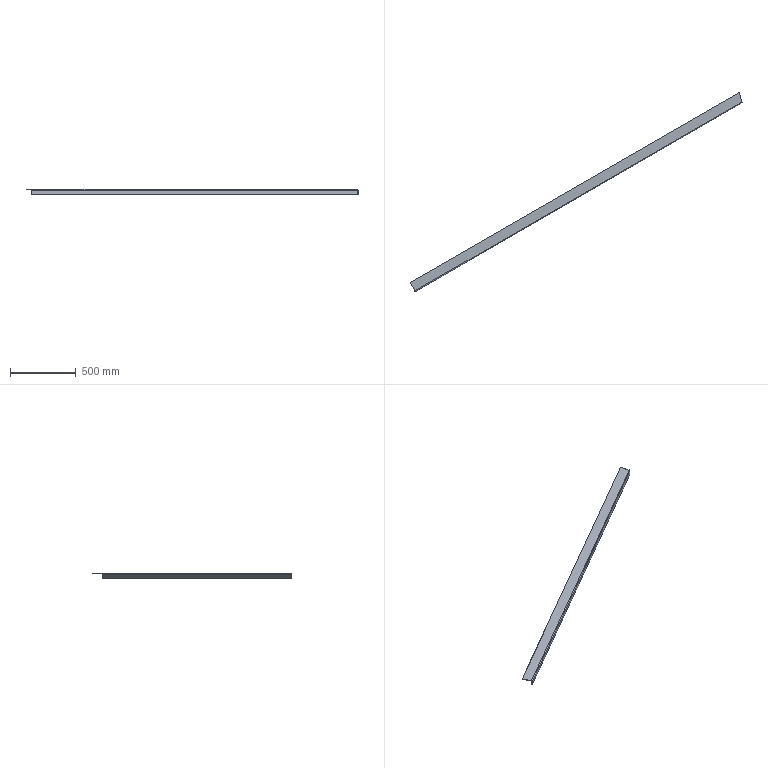Part | SolidWorks | features EdgeFlange 1, FlatPattern 1, ICE 1, SMBaseFlange 1, SheetMetal 1 | 1 solid | 16 faces | box 2517 x 1510 x 40 mm | volume 989838 mm3 | plane 14 | cylinder 2 | commonest cylinder face diameters 6 x1 12 x1
STEP:
#1=CARTESIAN_POINT('',(-2.01,7.5,-3.));
#2=VERTEX_POINT('',#1);
#3=CARTESIAN_POINT('',(-2.01,7.5,0.));
#4=VERTEX_POINT('',#3);
#5=CARTESIAN_POINT('',(-2.01,7.5,-3.));
#6=DIRECTION('',(0.,0.,1.));
#7=VECTOR('',#6,1000.);
#8=LINE('',#5,#7);
#9=EDGE_CURVE('',#2,#4,#8,.T.);
#10=ORIENTED_EDGE('',*,*,#9,.F.);
#11=CARTESIAN_POINT('',(-21.436,80.,-3.));
#12=VERTEX_POINT('',#11);
#13=CARTESIAN_POINT('',(0.,0.,-3.));
#14=DIRECTION('',(-0.2588,0.9659,0.));
#15=VECTOR('',#14,1000.);
#16=LINE('',#13,#15);
#17=EDGE_CURVE('',#2,#12,#16,.T.);
#18=ORIENTED_EDGE('',*,*,#17,.T.);
#19=CARTESIAN_POINT('',(-21.436,80.,0.));
#20=VERTEX_POINT('',#19);
#21=CARTESIAN_POINT('',(-21.436,80.,-3.));
#22=DIRECTION('',(0.,0.,1.));
#23=VECTOR('',#22,1000.);
#24=LINE('',#21,#23);
#25=EDGE_CURVE('',#12,#20,#24,.T.);
#26=ORIENTED_EDGE('',*,*,#25,.T.);
#27=CARTESIAN_POINT('',(0.,0.,0.));
#28=DIRECTION('',(-0.2588,0.9659,0.));
#29=VECTOR('',#28,1000.);
#30=LINE('',#27,#29);
#31=EDGE_CURVE('',#4,#20,#30,.T.);
#32=ORIENTED_EDGE('',*,*,#31,.F.);
#33=EDGE_LOOP('',(#10,#18,#26,#32));
#34=FACE_OUTER_BOUND('',#33,.T.);
#35=CARTESIAN_POINT('',(0.,0.,-3.));
#36=DIRECTION('',(0.9659,0.2588,0.));
#37=DIRECTION('',(-0.2588,0.9659,0.));
#38=AXIS2_PLACEMENT_3D('',#35,#36,#37);
#39=PLANE('',#38);
#40=ADVANCED_FACE('',(#34),#39,.T.);
#41=CARTESIAN_POINT('',(-2516.833,-1360.718,-3.));
#42=VERTEX_POINT('',#41);
#43=CARTESIAN_POINT('',(-2479.833,-1424.804,-3.));
#44=VERTEX_POINT('',#43);
#45=CARTESIAN_POINT('',(-2476.833,-1430.,-3.));
#46=DIRECTION('',(0.5,-0.866,0.));
#47=VECTOR('',#46,1000.);
#48=LINE('',#45,#47);
#49=EDGE_CURVE('',#42,#44,#48,.T.);
#50=ORIENTED_EDGE('',*,*,#49,.T.);
#51=CARTESIAN_POINT('',(-2479.833,-1424.804,0.));
#52=VERTEX_POINT('',#51);
#53=CARTESIAN_POINT('',(-2479.833,-1424.804,-3.));
#54=DIRECTION('',(0.,0.,1.));
#55=VECTOR('',#54,1000.);
#56=LINE('',#53,#55);
#57=EDGE_CURVE('',#44,#52,#56,.T.);
#58=ORIENTED_EDGE('',*,*,#57,.T.);
#59=CARTESIAN_POINT('',(-2516.833,-1360.718,0.));
#60=VERTEX_POINT('',#59);
#61=CARTESIAN_POINT('',(-2476.833,-1430.,0.));
#62=DIRECTION('',(0.5,-0.866,0.));
#63=VECTOR('',#62,1000.);
#64=LINE('',#61,#63);
#65=EDGE_CURVE('',#60,#52,#64,.T.);
#66=ORIENTED_EDGE('',*,*,#65,.F.);
#67=CARTESIAN_POINT('',(-2516.833,-1360.718,-3.));
#68=DIRECTION('',(0.,0.,1.));
#69=VECTOR('',#68,1000.);
#70=LINE('',#67,#69);
#71=EDGE_CURVE('',#42,#60,#70,.T.);
#72=ORIENTED_EDGE('',*,*,#71,.F.);
#73=EDGE_LOOP('',(#50,#58,#66,#72));
#74=FACE_OUTER_BOUND('',#73,.T.);
#75=CARTESIAN_POINT('',(-2476.833,-1430.,-3.));
#76=DIRECTION('',(-0.866,-0.5,0.));
#77=DIRECTION('',(0.5,-0.866,0.));
#78=AXIS2_PLACEMENT_3D('',#75,#76,#77);
#79=PLANE('',#78);
#80=ADVANCED_FACE('',(#74),#79,.T.);
#81=ORIENTED_EDGE('',*,*,#17,.F.);
#82=CARTESIAN_POINT('',(-3.75,6.495,-3.));
#83=VERTEX_POINT('',#82);
#84=CARTESIAN_POINT('',(-3.75,6.495,-3.));
#85=DIRECTION('',(0.866,0.5,0.));
#86=VECTOR('',#85,1000.);
#87=LINE('',#84,#86);
#88=EDGE_CURVE('',#83,#2,#87,.T.);
#89=ORIENTED_EDGE('',*,*,#88,.F.);
#90=CARTESIAN_POINT('',(-3.,5.196,-3.));
#91=VERTEX_POINT('',#90);
#92=CARTESIAN_POINT('',(-3.,5.196,-3.));
#93=DIRECTION('',(-0.5,0.866,0.));
#94=VECTOR('',#93,1000.);
#95=LINE('',#92,#94);
#96=EDGE_CURVE('',#91,#83,#95,.T.);
#97=ORIENTED_EDGE('',*,*,#96,.F.);
#98=CARTESIAN_POINT('',(-2479.833,-1424.804,-3.));
#99=DIRECTION('',(0.866,0.5,0.));
#100=VECTOR('',#99,1000.);
#101=LINE('',#98,#100);
#102=EDGE_CURVE('',#44,#91,#101,.T.);
#103=ORIENTED_EDGE('',*,*,#102,.F.);
#104=ORIENTED_EDGE('',*,*,#49,.F.);
#105=CARTESIAN_POINT('',(-21.436,80.,-3.));
#106=DIRECTION('',(-0.866,-0.5,0.));
#107=VECTOR('',#106,1000.);
#108=LINE('',#105,#107);
#109=EDGE_CURVE('',#12,#42,#108,.T.);
#110=ORIENTED_EDGE('',*,*,#109,.F.);
#111=EDGE_LOOP('',(#81,#89,#97,#103,#104,#110));
#112=FACE_OUTER_BOUND('',#111,.T.);
#113=CARTESIAN_POINT('',(0.,0.,-3.));
#114=DIRECTION('',(0.,0.,1.));
#115=DIRECTION('',(1.,0.,0.));
#116=AXIS2_PLACEMENT_3D('',#113,#114,#115);
#117=PLANE('',#116);
#118=ADVANCED_FACE('',(#112),#117,.F.);
#119=CARTESIAN_POINT('',(-3.75,6.495,0.));
#120=VERTEX_POINT('',#119);
#121=CARTESIAN_POINT('',(-3.75,6.495,0.));
#122=DIRECTION('',(0.866,0.5,0.));
#123=VECTOR('',#122,1000.);
#124=LINE('',#121,#123);
#125=EDGE_CURVE('',#120,#4,#124,.T.);
#126=ORIENTED_EDGE('',*,*,#125,.T.);
#127=ORIENTED_EDGE('',*,*,#31,.T.);
#128=CARTESIAN_POINT('',(-21.436,80.,0.));
#129=DIRECTION('',(-0.866,-0.5,0.));
#130=VECTOR('',#129,1000.);
#131=LINE('',#128,#130);
#132=EDGE_CURVE('',#20,#60,#131,.T.);
#133=ORIENTED_EDGE('',*,*,#132,.T.);
#134=ORIENTED_EDGE('',*,*,#65,.T.);
#135=CARTESIAN_POINT('',(-3.,5.196,0.));
#136=VERTEX_POINT('',#135);
#137=CARTESIAN_POINT('',(-2479.833,-1424.804,0.));
#138=DIRECTION('',(0.866,0.5,0.));
#139=VECTOR('',#138,1000.);
#140=LINE('',#137,#139);
#141=EDGE_CURVE('',#52,#136,#140,.T.);
#142=ORIENTED_EDGE('',*,*,#141,.T.);
#143=CARTESIAN_POINT('',(0.,0.,0.));
#144=DIRECTION('',(-0.5,0.866,0.));
#145=VECTOR('',#144,1000.);
#146=LINE('',#143,#145);
#147=EDGE_CURVE('',#136,#120,#146,.T.);
#148=ORIENTED_EDGE('',*,*,#147,.T.);
#149=EDGE_LOOP('',(#126,#127,#133,#134,#142,#148));
#150=FACE_OUTER_BOUND('',#149,.T.);
#151=CARTESIAN_POINT('',(0.,0.,0.));
#152=DIRECTION('',(0.,0.,1.));
#153=DIRECTION('',(1.,0.,0.));
#154=AXIS2_PLACEMENT_3D('',#151,#152,#153);
#155=PLANE('',#154);
#156=ADVANCED_FACE('',(#150),#155,.T.);
#157=ORIENTED_EDGE('',*,*,#132,.F.);
#158=ORIENTED_EDGE('',*,*,#25,.F.);
#159=ORIENTED_EDGE('',*,*,#109,.T.);
#160=ORIENTED_EDGE('',*,*,#71,.T.);
#161=EDGE_LOOP('',(#157,#158,#159,#160));
#162=FACE_OUTER_BOUND('',#161,.T.);
#163=CARTESIAN_POINT('',(-21.436,80.,-3.));
#164=DIRECTION('',(-0.5,0.866,0.));
#165=DIRECTION('',(-0.866,-0.5,0.));
#166=AXIS2_PLACEMENT_3D('',#163,#164,#165);
#167=PLANE('',#166);
#168=ADVANCED_FACE('',(#162),#167,.T.);
#169=ORIENTED_EDGE('',*,*,#147,.F.);
#170=CARTESIAN_POINT('',(-3.,5.196,-3.));
#171=DIRECTION('',(0.,0.,1.));
#172=VECTOR('',#171,1000.);
#173=LINE('',#170,#172);
#174=EDGE_CURVE('',#91,#136,#173,.T.);
#175=ORIENTED_EDGE('',*,*,#174,.F.);
#176=ORIENTED_EDGE('',*,*,#96,.T.);
#177=CARTESIAN_POINT('',(-3.75,6.495,-3.));
#178=DIRECTION('',(0.,0.,1.));
#179=VECTOR('',#178,1000.);
#180=LINE('',#177,#179);
#181=EDGE_CURVE('',#83,#120,#180,.T.);
#182=ORIENTED_EDGE('',*,*,#181,.T.);
#183=EDGE_LOOP('',(#169,#175,#176,#182));
#184=FACE_OUTER_BOUND('',#183,.T.);
#185=CARTESIAN_POINT('',(-3.,5.196,-3.));
#186=DIRECTION('',(0.866,0.5,0.));
#187=DIRECTION('',(-0.5,0.866,0.));
#188=AXIS2_PLACEMENT_3D('',#185,#186,#187);
#189=PLANE('',#188);
#190=ADVANCED_FACE('',(#184),#189,.T.);
#191=ORIENTED_EDGE('',*,*,#125,.F.);
#192=ORIENTED_EDGE('',*,*,#181,.F.);
#193=ORIENTED_EDGE('',*,*,#88,.T.);
#194=ORIENTED_EDGE('',*,*,#9,.T.);
#195=EDGE_LOOP('',(#191,#192,#193,#194));
#196=FACE_OUTER_BOUND('',#195,.T.);
#197=CARTESIAN_POINT('',(-3.75,6.495,-3.));
#198=DIRECTION('',(0.5,-0.866,0.));
#199=DIRECTION('',(0.866,0.5,0.));
#200=AXIS2_PLACEMENT_3D('',#197,#198,#199);
#201=PLANE('',#200);
#202=ADVANCED_FACE('',(#196),#201,.T.);
#203=CARTESIAN_POINT('',(-1.5,2.598,-6.));
#204=VERTEX_POINT('',#203);
#205=CARTESIAN_POINT('',(0.,0.,-6.));
#206=VERTEX_POINT('',#205);
#207=CARTESIAN_POINT('',(0.,0.,-6.));
#208=DIRECTION('',(0.5,-0.866,0.));
#209=VECTOR('',#208,1000.);
#210=LINE('',#207,#209);
#211=EDGE_CURVE('',#204,#206,#210,.T.);
#212=ORIENTED_EDGE('',*,*,#211,.F.);
#213=CARTESIAN_POINT('',(-3.,5.196,-6.));
#214=DIRECTION('',(0.866,0.5,0.));
#215=DIRECTION('',(0.5,-0.866,0.));
#216=AXIS2_PLACEMENT_3D('',#213,#214,#215);
#217=CIRCLE('',#216,3.);
#218=EDGE_CURVE('',#91,#204,#217,.T.);
#219=ORIENTED_EDGE('',*,*,#218,.F.);
#220=ORIENTED_EDGE('',*,*,#174,.T.);
#221=CARTESIAN_POINT('',(-3.,5.196,-6.));
#222=DIRECTION('',(0.866,0.5,0.));
#223=DIRECTION('',(0.5,-0.866,0.));
#224=AXIS2_PLACEMENT_3D('',#221,#222,#223);
#225=CIRCLE('',#224,6.);
#226=EDGE_CURVE('',#136,#206,#225,.T.);
#227=ORIENTED_EDGE('',*,*,#226,.T.);
#228=EDGE_LOOP('',(#212,#219,#220,#227));
#229=FACE_OUTER_BOUND('',#228,.T.);
#230=CARTESIAN_POINT('',(-3.,5.196,-6.));
#231=DIRECTION('',(0.866,0.5,0.));
#232=DIRECTION('',(-0.5,0.866,0.));
#233=AXIS2_PLACEMENT_3D('',#230,#231,#232);
#234=PLANE('',#233);
#235=ADVANCED_FACE('',(#229),#234,.T.);
#236=CARTESIAN_POINT('',(-2478.333,-1427.402,-6.));
#237=VERTEX_POINT('',#236);
#238=CARTESIAN_POINT('',(-2479.833,-1424.804,-6.));
#239=DIRECTION('',(-0.866,-0.5,0.));
#240=DIRECTION('',(0.5,-0.866,0.));
#241=AXIS2_PLACEMENT_3D('',#238,#239,#240);
#242=CIRCLE('',#241,3.);
#243=EDGE_CURVE('',#237,#44,#242,.T.);
#244=ORIENTED_EDGE('',*,*,#243,.F.);
#245=CARTESIAN_POINT('',(-2476.833,-1430.,-6.));
#246=VERTEX_POINT('',#245);
#247=CARTESIAN_POINT('',(-2478.333,-1427.402,-6.));
#248=DIRECTION('',(0.5,-0.866,0.));
#249=VECTOR('',#248,1000.);
#250=LINE('',#247,#249);
#251=EDGE_CURVE('',#237,#246,#250,.T.);
#252=ORIENTED_EDGE('',*,*,#251,.T.);
#253=CARTESIAN_POINT('',(-2479.833,-1424.804,-6.));
#254=DIRECTION('',(-0.866,-0.5,0.));
#255=DIRECTION('',(0.5,-0.866,0.));
#256=AXIS2_PLACEMENT_3D('',#253,#254,#255);
#257=CIRCLE('',#256,6.);
#258=EDGE_CURVE('',#246,#52,#257,.T.);
#259=ORIENTED_EDGE('',*,*,#258,.T.);
#260=ORIENTED_EDGE('',*,*,#57,.F.);
#261=EDGE_LOOP('',(#244,#252,#259,#260));
#262=FACE_OUTER_BOUND('',#261,.T.);
#263=CARTESIAN_POINT('',(-2479.833,-1424.804,-6.));
#264=DIRECTION('',(0.866,0.5,0.));
#265=DIRECTION('',(-0.5,0.866,0.));
#266=AXIS2_PLACEMENT_3D('',#263,#264,#265);
#267=PLANE('',#266);
#268=ADVANCED_FACE('',(#262),#267,.F.);
#269=ORIENTED_EDGE('',*,*,#141,.F.);
#270=ORIENTED_EDGE('',*,*,#258,.F.);
#271=CARTESIAN_POINT('',(0.,0.,-6.));
#272=DIRECTION('',(-0.866,-0.5,0.));
#273=VECTOR('',#272,1000.);
#274=LINE('',#271,#273);
#275=EDGE_CURVE('',#206,#246,#274,.T.);
#276=ORIENTED_EDGE('',*,*,#275,.F.);
#277=ORIENTED_EDGE('',*,*,#226,.F.);
#278=EDGE_LOOP('',(#269,#270,#276,#277));
#279=FACE_OUTER_BOUND('',#278,.T.);
#280=CARTESIAN_POINT('',(-2479.833,-1424.804,-6.));
#281=DIRECTION('',(-0.866,-0.5,0.));
#282=DIRECTION('',(0.5,-0.866,0.));
#283=AXIS2_PLACEMENT_3D('',#280,#281,#282);
#284=CYLINDRICAL_SURFACE('',#283,6.);
#285=ADVANCED_FACE('',(#279),#284,.T.);
#286=ORIENTED_EDGE('',*,*,#102,.T.);
#287=ORIENTED_EDGE('',*,*,#218,.T.);
#288=CARTESIAN_POINT('',(-1.5,2.598,-6.));
#289=DIRECTION('',(-0.866,-0.5,0.));
#290=VECTOR('',#289,1000.);
#291=LINE('',#288,#290);
#292=EDGE_CURVE('',#204,#237,#291,.T.);
#293=ORIENTED_EDGE('',*,*,#292,.T.);
#294=ORIENTED_EDGE('',*,*,#243,.T.);
#295=EDGE_LOOP('',(#286,#287,#293,#294));
#296=FACE_OUTER_BOUND('',#295,.T.);
#297=CARTESIAN_POINT('',(-2479.833,-1424.804,-6.));
#298=DIRECTION('',(-0.866,-0.5,0.));
#299=DIRECTION('',(0.5,-0.866,0.));
#300=AXIS2_PLACEMENT_3D('',#297,#298,#299);
#301=CYLINDRICAL_SURFACE('',#300,3.);
#302=ADVANCED_FACE('',(#296),#301,.F.);
#303=CARTESIAN_POINT('',(-2476.833,-1430.,-40.));
#304=VERTEX_POINT('',#303);
#305=CARTESIAN_POINT('',(-2476.833,-1430.,-3.));
#306=DIRECTION('',(0.,0.,1.));
#307=VECTOR('',#306,1000.);
#308=LINE('',#305,#307);
#309=EDGE_CURVE('',#304,#246,#308,.T.);
#310=ORIENTED_EDGE('',*,*,#309,.T.);
#311=ORIENTED_EDGE('',*,*,#251,.F.);
#312=CARTESIAN_POINT('',(-2478.333,-1427.402,-40.));
#313=VERTEX_POINT('',#312);
#314=CARTESIAN_POINT('',(-2478.333,-1427.402,0.));
#315=DIRECTION('',(0.,0.,1.));
#316=VECTOR('',#315,1000.);
#317=LINE('',#314,#316);
#318=EDGE_CURVE('',#313,#237,#317,.T.);
#319=ORIENTED_EDGE('',*,*,#318,.F.);
#320=CARTESIAN_POINT('',(-2476.833,-1430.,-40.));
#321=DIRECTION('',(-0.5,0.866,0.));
#322=VECTOR('',#321,1000.);
#323=LINE('',#320,#322);
#324=EDGE_CURVE('',#304,#313,#323,.T.);
#325=ORIENTED_EDGE('',*,*,#324,.F.);
#326=EDGE_LOOP('',(#310,#311,#319,#325));
#327=FACE_OUTER_BOUND('',#326,.T.);
#328=CARTESIAN_POINT('',(-2476.833,-1430.,-3.));
#329=DIRECTION('',(-0.866,-0.5,0.));
#330=DIRECTION('',(0.5,-0.866,0.));
#331=AXIS2_PLACEMENT_3D('',#328,#329,#330);
#332=PLANE('',#331);
#333=ADVANCED_FACE('',(#327),#332,.T.);
#334=CARTESIAN_POINT('',(-1.5,2.598,-40.));
#335=VERTEX_POINT('',#334);
#336=CARTESIAN_POINT('',(-1.5,2.598,0.));
#337=DIRECTION('',(0.,0.,-1.));
#338=VECTOR('',#337,1000.);
#339=LINE('',#336,#338);
#340=EDGE_CURVE('',#204,#335,#339,.T.);
#341=ORIENTED_EDGE('',*,*,#340,.F.);
#342=ORIENTED_EDGE('',*,*,#211,.T.);
#343=CARTESIAN_POINT('',(0.,0.,-40.));
#344=VERTEX_POINT('',#343);
#345=CARTESIAN_POINT('',(0.,0.,-40.));
#346=DIRECTION('',(0.,0.,-1.));
#347=VECTOR('',#346,1000.);
#348=LINE('',#345,#347);
#349=EDGE_CURVE('',#206,#344,#348,.T.);
#350=ORIENTED_EDGE('',*,*,#349,.T.);
#351=CARTESIAN_POINT('',(0.,0.,-40.));
#352=DIRECTION('',(-0.5,0.866,0.));
#353=VECTOR('',#352,1000.);
#354=LINE('',#351,#353);
#355=EDGE_CURVE('',#344,#335,#354,.T.);
#356=ORIENTED_EDGE('',*,*,#355,.T.);
#357=EDGE_LOOP('',(#341,#342,#350,#356));
#358=FACE_OUTER_BOUND('',#357,.T.);
#359=CARTESIAN_POINT('',(0.,0.,-40.));
#360=DIRECTION('',(0.866,0.5,0.));
#361=DIRECTION('',(-0.5,0.866,0.));
#362=AXIS2_PLACEMENT_3D('',#359,#360,#361);
#363=PLANE('',#362);
#364=ADVANCED_FACE('',(#358),#363,.T.);
#365=ORIENTED_EDGE('',*,*,#349,.F.);
#366=ORIENTED_EDGE('',*,*,#275,.T.);
#367=ORIENTED_EDGE('',*,*,#309,.F.);
#368=CARTESIAN_POINT('',(-2476.833,-1430.,-40.));
#369=DIRECTION('',(-0.866,-0.5,0.));
#370=VECTOR('',#369,1000.);
#371=LINE('',#368,#370);
#372=EDGE_CURVE('',#344,#304,#371,.T.);
#373=ORIENTED_EDGE('',*,*,#372,.F.);
#374=EDGE_LOOP('',(#365,#366,#367,#373));
#375=FACE_OUTER_BOUND('',#374,.T.);
#376=CARTESIAN_POINT('',(0.,0.,0.));
#377=DIRECTION('',(0.5,-0.866,0.));
#378=DIRECTION('',(0.866,0.5,0.));
#379=AXIS2_PLACEMENT_3D('',#376,#377,#378);
#380=PLANE('',#379);
#381=ADVANCED_FACE('',(#375),#380,.T.);
#382=ORIENTED_EDGE('',*,*,#292,.F.);
#383=ORIENTED_EDGE('',*,*,#340,.T.);
#384=CARTESIAN_POINT('',(-1.5,2.598,-40.));
#385=DIRECTION('',(-0.866,-0.5,0.));
#386=VECTOR('',#385,1000.);
#387=LINE('',#384,#386);
#388=EDGE_CURVE('',#335,#313,#387,.T.);
#389=ORIENTED_EDGE('',*,*,#388,.T.);
#390=ORIENTED_EDGE('',*,*,#318,.T.);
#391=EDGE_LOOP('',(#382,#383,#389,#390));
#392=FACE_OUTER_BOUND('',#391,.T.);
#393=CARTESIAN_POINT('',(-1.5,2.598,0.));
#394=DIRECTION('',(0.5,-0.866,0.));
#395=DIRECTION('',(0.866,0.5,0.));
#396=AXIS2_PLACEMENT_3D('',#393,#394,#395);
#397=PLANE('',#396);
#398=ADVANCED_FACE('',(#392),#397,.F.);
#399=ORIENTED_EDGE('',*,*,#388,.F.);
#400=ORIENTED_EDGE('',*,*,#355,.F.);
#401=ORIENTED_EDGE('',*,*,#372,.T.);
#402=ORIENTED_EDGE('',*,*,#324,.T.);
#403=EDGE_LOOP('',(#399,#400,#401,#402));
#404=FACE_OUTER_BOUND('',#403,.T.);
#405=CARTESIAN_POINT('',(-2476.833,-1430.,-40.));
#406=DIRECTION('',(0.,0.,-1.));
#407=DIRECTION('',(0.,1.,0.));
#408=AXIS2_PLACEMENT_3D('',#405,#406,#407);
#409=PLANE('',#408);
#410=ADVANCED_FACE('',(#404),#409,.T.);
#411=CLOSED_SHELL('',(#40,#80,#118,#156,#168,#190,#202,#235,#268,#285,#302,#333,#364,#381,#398,#410));
#412=MANIFOLD_SOLID_BREP('',#411);
#413=CARTESIAN_POINT('',(0.,0.,0.));
#414=DIRECTION('',(0.,0.,1.));
#415=DIRECTION('',(1.,0.,0.));
#416=AXIS2_PLACEMENT_3D('',#413,#414,#415);
#417=(LENGTH_UNIT()NAMED_UNIT(*)SI_UNIT(.MILLI.,.METRE.));
#418=UNCERTAINTY_MEASURE_WITH_UNIT(LENGTH_MEASURE(0.00001),#417,'','');
#419=(NAMED_UNIT(*)PLANE_ANGLE_UNIT()SI_UNIT($,.RADIAN.));
#420=(NAMED_UNIT(*)SI_UNIT($,.STERADIAN.)SOLID_ANGLE_UNIT());
#421=(GEOMETRIC_REPRESENTATION_CONTEXT(3)GLOBAL_UNCERTAINTY_ASSIGNED_CONTEXT((#418))GLOBAL_UNIT_ASSIGNED_CONTEXT((#417,#419,#420))REPRESENTATION_CONTEXT('',''));
#422=ADVANCED_BREP_SHAPE_REPRESENTATION('',(#412,#416),#421);